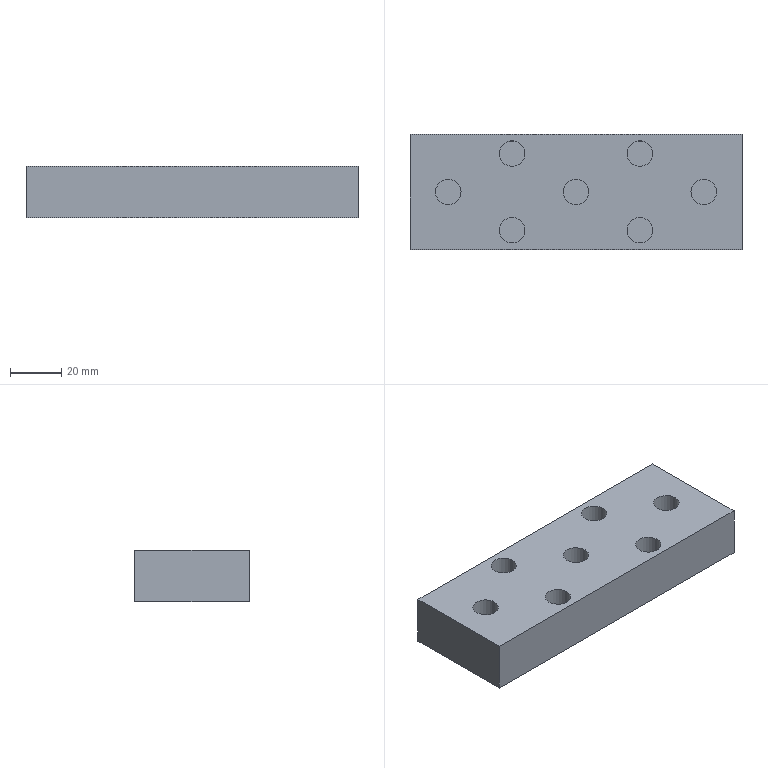CAM job | NX | 3-axis milling, drilling | part box 130 x 45 x 20 mm | stock box 135 x 50 x 20 mm
Tools:
number,name,description,diameter,corner_radius,flute_length,length,flutes
2,D10点钻,定心钻D10,10.0,0.0,87.0,133.0,2
9,D8开粗,D8,8.0,0.0,20.0,60.0,2
10,D8精光,D8,8.0,0.0,20.0,60.0,2
7,D10开粗,D10,10.0,0.0,25.0,75.0,2
1,D63R0.8,方肩铣刀片,63.0,0.8,15.0,80.0,2
4,Z6.5,Z6.5直柄钻头,6.5,0.0,63.0,101.0,2
Operations:
program,operation,operation_type,tool,method,geometry_group,spindle_rpm,surface_speed,feed_per_tooth,feed_cut,feed_plunge,cut_length_mm,path_length_mm,cut_time_min,machine_time_min
XX-CNC1,PLANAR_MILL,PlanarMilling,D63R0.8,METHOD,MCS_1,3500.0,100.0,0.1178,800.0,100.0,262.0,316.0,0.3275,0.3329
XX-CNC1,ADAPTIVE_MILLING,CavityMilling,D10开粗,METHOD,W1,5500.0,100.0,0.1178,2500.0,100.0,2275.601,2369.601,0.7864,0.7958
XX-CNC1,DRILLING,Operation,D10点钻,METHOD,W1,2000.0,0.0,0.0,200.0,0.0,31.5,318.534,0.1575,0.1862
XX-CNC1,DRILLING_COPY,Operation,Z6.5,METHOD,W1,3000.0,0.0,0.0,200.0,0.0,91.0,437.534,0.455,0.4897
XX-CNC1,PLANAR_MILL_1,PlanarMilling,D8开粗,METHOD,W1,4500.0,100.0,0.1178,800.0,100.0,1517.848,2167.321,1.897,1.962
XX-CNC1,PLANAR_MILL_1_COPY,PlanarMilling,D8精光,METHOD,W1,4500.0,100.0,0.1178,600.0,100.0,156.574,864.103,0.261,0.3317
XX-CNC1,PLANAR_MILL_2,PlanarMilling,D8精光,METHOD,W1,4500.0,100.0,0.1178,600.0,100.0,388.706,482.706,0.6478,0.6572
XX-CNC1,PLANAR_MILL_1_COPY_COPY,PlanarMilling,D10点钻,METHOD,W1,3500.0,100.0,0.1178,800.0,100.0,200.706,788.7,0.2509,0.3097
XX-CNC1,PLANAR_MILL_2_COPY,PlanarMilling,D10点钻,METHOD,W1,3500.0,100.0,0.1178,800.0,100.0,374.625,431.625,0.4683,0.474